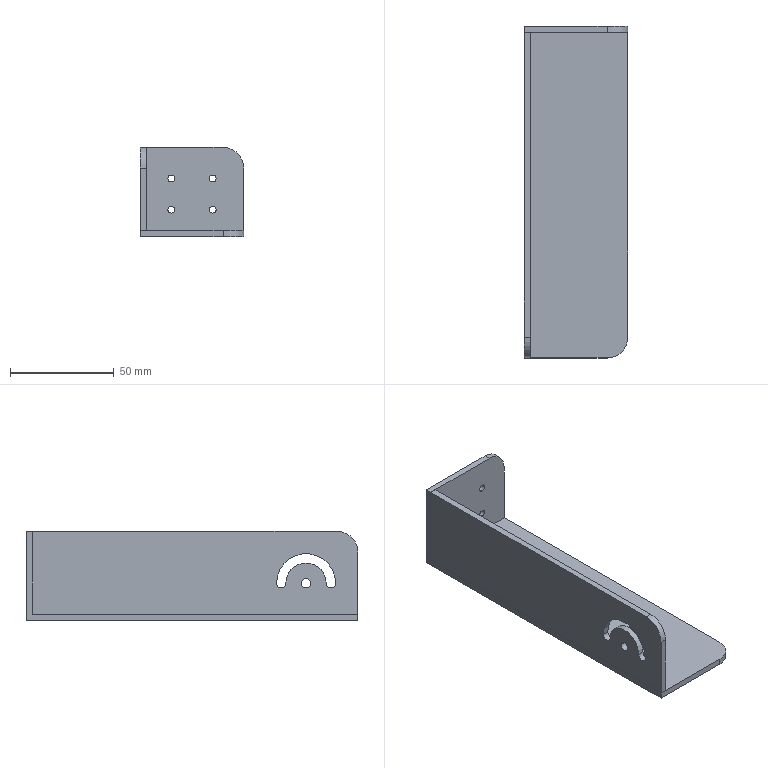Part | SolidWorks | features ICE 3, Fillet 2, Extrusion 1, HoleWzd 1 | 2 solids | 31 faces | box 50 x 160 x 43 mm | volume 47940 mm3 | cylinder 17 | plane 14 | commonest cylinder face diameters 3.3 x8 4.5 x4 20 x3 19.5 x1 28.5 x1
STEP:
#1=CARTESIAN_POINT('',(-25.,-52.75,18.));
#2=VERTEX_POINT('',#1);
#3=CARTESIAN_POINT('',(-25.,-57.25,18.));
#4=VERTEX_POINT('',#3);
#5=CARTESIAN_POINT('',(-25.,-55.,18.));
#6=DIRECTION('',(-1.,0.,0.));
#7=DIRECTION('',(0.,-1.,0.));
#8=AXIS2_PLACEMENT_3D('',#5,#6,#7);
#9=CIRCLE('',#8,2.25);
#10=EDGE_CURVE('',#2,#4,#9,.T.);
#11=ORIENTED_EDGE('',*,*,#10,.T.);
#12=CARTESIAN_POINT('',(-22.,-57.25,18.));
#13=VERTEX_POINT('',#12);
#14=CARTESIAN_POINT('',(-32.,-57.25,18.));
#15=DIRECTION('',(1.,0.,0.));
#16=VECTOR('',#15,1000.);
#17=LINE('',#14,#16);
#18=EDGE_CURVE('',#4,#13,#17,.T.);
#19=ORIENTED_EDGE('',*,*,#18,.T.);
#20=CARTESIAN_POINT('',(-22.,-52.75,18.));
#21=VERTEX_POINT('',#20);
#22=CARTESIAN_POINT('',(-22.,-55.,18.));
#23=DIRECTION('',(1.,0.,0.));
#24=DIRECTION('',(0.,1.,0.));
#25=AXIS2_PLACEMENT_3D('',#22,#23,#24);
#26=CIRCLE('',#25,2.25);
#27=EDGE_CURVE('',#13,#21,#26,.T.);
#28=ORIENTED_EDGE('',*,*,#27,.T.);
#29=CARTESIAN_POINT('',(-32.,-52.75,18.));
#30=DIRECTION('',(1.,0.,0.));
#31=VECTOR('',#30,1000.);
#32=LINE('',#29,#31);
#33=EDGE_CURVE('',#2,#21,#32,.T.);
#34=ORIENTED_EDGE('',*,*,#33,.F.);
#35=EDGE_LOOP('',(#11,#19,#28,#34));
#36=FACE_OUTER_BOUND('',#35,.T.);
#37=CARTESIAN_POINT('',(-32.,-55.,18.));
#38=DIRECTION('',(1.,0.,0.));
#39=DIRECTION('',(0.,1.,0.));
#40=AXIS2_PLACEMENT_3D('',#37,#38,#39);
#41=CYLINDRICAL_SURFACE('',#40,2.25);
#42=ADVANCED_FACE('',(#36),#41,.F.);
#43=CARTESIAN_POINT('',(-22.,-55.,18.));
#44=DIRECTION('',(1.,0.,0.));
#45=DIRECTION('',(0.,1.,0.));
#46=AXIS2_PLACEMENT_3D('',#43,#44,#45);
#47=CIRCLE('',#46,2.25);
#48=EDGE_CURVE('',#21,#13,#47,.T.);
#49=ORIENTED_EDGE('',*,*,#48,.F.);
#50=ORIENTED_EDGE('',*,*,#27,.F.);
#51=EDGE_LOOP('',(#49,#50));
#52=FACE_BOUND('',#51,.T.);
#53=CARTESIAN_POINT('',(-22.,-70.,43.));
#54=VERTEX_POINT('',#53);
#55=CARTESIAN_POINT('',(-22.,77.,43.));
#56=VERTEX_POINT('',#55);
#57=CARTESIAN_POINT('',(-22.,77.,43.));
#58=DIRECTION('',(0.,1.,0.));
#59=VECTOR('',#58,1000.);
#60=LINE('',#57,#59);
#61=EDGE_CURVE('',#54,#56,#60,.T.);
#62=ORIENTED_EDGE('',*,*,#61,.F.);
#63=CARTESIAN_POINT('',(-22.,-80.,33.));
#64=VERTEX_POINT('',#63);
#65=CARTESIAN_POINT('',(-22.,-70.,33.));
#66=DIRECTION('',(1.,0.,0.));
#67=DIRECTION('',(0.,-1.,0.));
#68=AXIS2_PLACEMENT_3D('',#65,#66,#67);
#69=CIRCLE('',#68,10.);
#70=EDGE_CURVE('',#54,#64,#69,.T.);
#71=ORIENTED_EDGE('',*,*,#70,.T.);
#72=CARTESIAN_POINT('',(-22.,-80.,3.));
#73=VERTEX_POINT('',#72);
#74=CARTESIAN_POINT('',(-22.,-80.,3.));
#75=DIRECTION('',(0.,0.,1.));
#76=VECTOR('',#75,1000.);
#77=LINE('',#74,#76);
#78=EDGE_CURVE('',#73,#64,#77,.T.);
#79=ORIENTED_EDGE('',*,*,#78,.F.);
#80=CARTESIAN_POINT('',(-22.,77.,3.));
#81=VERTEX_POINT('',#80);
#82=CARTESIAN_POINT('',(-22.,77.,3.));
#83=DIRECTION('',(0.,-1.,0.));
#84=VECTOR('',#83,1000.);
#85=LINE('',#82,#84);
#86=EDGE_CURVE('',#81,#73,#85,.T.);
#87=ORIENTED_EDGE('',*,*,#86,.F.);
#88=CARTESIAN_POINT('',(-22.,77.,3.));
#89=DIRECTION('',(0.,0.,-1.));
#90=VECTOR('',#89,1000.);
#91=LINE('',#88,#90);
#92=EDGE_CURVE('',#56,#81,#91,.T.);
#93=ORIENTED_EDGE('',*,*,#92,.F.);
#94=EDGE_LOOP('',(#62,#71,#79,#87,#93));
#95=FACE_OUTER_BOUND('',#94,.T.);
#96=CARTESIAN_POINT('',(-22.,-64.75,18.));
#97=VERTEX_POINT('',#96);
#98=CARTESIAN_POINT('',(-22.,-45.25,18.));
#99=VERTEX_POINT('',#98);
#100=CARTESIAN_POINT('',(-22.,-55.,18.));
#101=DIRECTION('',(-1.,0.,0.));
#102=DIRECTION('',(0.,1.,0.));
#103=AXIS2_PLACEMENT_3D('',#100,#101,#102);
#104=CIRCLE('',#103,9.75);
#105=EDGE_CURVE('',#97,#99,#104,.T.);
#106=ORIENTED_EDGE('',*,*,#105,.F.);
#107=CARTESIAN_POINT('',(-22.,-69.25,18.));
#108=VERTEX_POINT('',#107);
#109=CARTESIAN_POINT('',(-22.,-67.,18.));
#110=DIRECTION('',(1.,0.,0.));
#111=DIRECTION('',(0.,1.,0.));
#112=AXIS2_PLACEMENT_3D('',#109,#110,#111);
#113=CIRCLE('',#112,2.25);
#114=EDGE_CURVE('',#108,#97,#113,.T.);
#115=ORIENTED_EDGE('',*,*,#114,.F.);
#116=CARTESIAN_POINT('',(-22.,-40.75,18.));
#117=VERTEX_POINT('',#116);
#118=CARTESIAN_POINT('',(-22.,-55.,18.));
#119=DIRECTION('',(1.,0.,0.));
#120=DIRECTION('',(0.,1.,0.));
#121=AXIS2_PLACEMENT_3D('',#118,#119,#120);
#122=CIRCLE('',#121,14.25);
#123=EDGE_CURVE('',#117,#108,#122,.T.);
#124=ORIENTED_EDGE('',*,*,#123,.F.);
#125=CARTESIAN_POINT('',(-22.,-43.,18.));
#126=DIRECTION('',(1.,0.,0.));
#127=DIRECTION('',(0.,1.,0.));
#128=AXIS2_PLACEMENT_3D('',#125,#126,#127);
#129=CIRCLE('',#128,2.25);
#130=EDGE_CURVE('',#99,#117,#129,.T.);
#131=ORIENTED_EDGE('',*,*,#130,.F.);
#132=EDGE_LOOP('',(#106,#115,#124,#131));
#133=FACE_BOUND('',#132,.T.);
#134=CARTESIAN_POINT('',(-22.,0.,0.));
#135=DIRECTION('',(-1.,0.,0.));
#136=DIRECTION('',(0.,-1.,0.));
#137=AXIS2_PLACEMENT_3D('',#134,#135,#136);
#138=PLANE('',#137);
#139=ADVANCED_FACE('',(#52,#95,#133),#138,.F.);
#140=CARTESIAN_POINT('',(-25.,-80.,3.));
#141=VERTEX_POINT('',#140);
#142=CARTESIAN_POINT('',(-25.,-80.,33.));
#143=VERTEX_POINT('',#142);
#144=CARTESIAN_POINT('',(-25.,-80.,3.));
#145=DIRECTION('',(0.,0.,1.));
#146=VECTOR('',#145,1000.);
#147=LINE('',#144,#146);
#148=EDGE_CURVE('',#141,#143,#147,.T.);
#149=ORIENTED_EDGE('',*,*,#148,.T.);
#150=CARTESIAN_POINT('',(-25.,-70.,43.));
#151=VERTEX_POINT('',#150);
#152=CARTESIAN_POINT('',(-25.,-70.,33.));
#153=DIRECTION('',(-1.,0.,0.));
#154=DIRECTION('',(0.,-1.,0.));
#155=AXIS2_PLACEMENT_3D('',#152,#153,#154);
#156=CIRCLE('',#155,10.);
#157=EDGE_CURVE('',#143,#151,#156,.T.);
#158=ORIENTED_EDGE('',*,*,#157,.T.);
#159=CARTESIAN_POINT('',(-25.,77.,43.));
#160=VERTEX_POINT('',#159);
#161=CARTESIAN_POINT('',(-25.,77.,43.));
#162=DIRECTION('',(0.,1.,0.));
#163=VECTOR('',#162,1000.);
#164=LINE('',#161,#163);
#165=EDGE_CURVE('',#151,#160,#164,.T.);
#166=ORIENTED_EDGE('',*,*,#165,.T.);
#167=CARTESIAN_POINT('',(-25.,77.,3.));
#168=VERTEX_POINT('',#167);
#169=CARTESIAN_POINT('',(-25.,77.,3.));
#170=DIRECTION('',(0.,0.,-1.));
#171=VECTOR('',#170,1000.);
#172=LINE('',#169,#171);
#173=EDGE_CURVE('',#160,#168,#172,.T.);
#174=ORIENTED_EDGE('',*,*,#173,.T.);
#175=CARTESIAN_POINT('',(-25.,77.,3.));
#176=DIRECTION('',(0.,-1.,0.));
#177=VECTOR('',#176,1000.);
#178=LINE('',#175,#177);
#179=EDGE_CURVE('',#168,#141,#178,.T.);
#180=ORIENTED_EDGE('',*,*,#179,.T.);
#181=EDGE_LOOP('',(#149,#158,#166,#174,#180));
#182=FACE_OUTER_BOUND('',#181,.T.);
#183=ORIENTED_EDGE('',*,*,#10,.F.);
#184=CARTESIAN_POINT('',(-25.,-55.,18.));
#185=DIRECTION('',(-1.,0.,0.));
#186=DIRECTION('',(0.,-1.,0.));
#187=AXIS2_PLACEMENT_3D('',#184,#185,#186);
#188=CIRCLE('',#187,2.25);
#189=EDGE_CURVE('',#4,#2,#188,.T.);
#190=ORIENTED_EDGE('',*,*,#189,.F.);
#191=EDGE_LOOP('',(#183,#190));
#192=FACE_BOUND('',#191,.T.);
#193=CARTESIAN_POINT('',(-25.,-64.75,18.));
#194=VERTEX_POINT('',#193);
#195=CARTESIAN_POINT('',(-25.,-69.25,18.));
#196=VERTEX_POINT('',#195);
#197=CARTESIAN_POINT('',(-25.,-67.,18.));
#198=DIRECTION('',(-1.,0.,0.));
#199=DIRECTION('',(0.,-1.,0.));
#200=AXIS2_PLACEMENT_3D('',#197,#198,#199);
#201=CIRCLE('',#200,2.25);
#202=EDGE_CURVE('',#194,#196,#201,.T.);
#203=ORIENTED_EDGE('',*,*,#202,.F.);
#204=CARTESIAN_POINT('',(-25.,-45.25,18.));
#205=VERTEX_POINT('',#204);
#206=CARTESIAN_POINT('',(-25.,-55.,18.));
#207=DIRECTION('',(1.,0.,0.));
#208=DIRECTION('',(0.,-1.,0.));
#209=AXIS2_PLACEMENT_3D('',#206,#207,#208);
#210=CIRCLE('',#209,9.75);
#211=EDGE_CURVE('',#205,#194,#210,.T.);
#212=ORIENTED_EDGE('',*,*,#211,.F.);
#213=CARTESIAN_POINT('',(-25.,-40.75,18.));
#214=VERTEX_POINT('',#213);
#215=CARTESIAN_POINT('',(-25.,-43.,18.));
#216=DIRECTION('',(-1.,0.,0.));
#217=DIRECTION('',(0.,-1.,0.));
#218=AXIS2_PLACEMENT_3D('',#215,#216,#217);
#219=CIRCLE('',#218,2.25);
#220=EDGE_CURVE('',#214,#205,#219,.T.);
#221=ORIENTED_EDGE('',*,*,#220,.F.);
#222=CARTESIAN_POINT('',(-25.,-55.,18.));
#223=DIRECTION('',(-1.,0.,0.));
#224=DIRECTION('',(0.,-1.,0.));
#225=AXIS2_PLACEMENT_3D('',#222,#223,#224);
#226=CIRCLE('',#225,14.25);
#227=EDGE_CURVE('',#196,#214,#226,.T.);
#228=ORIENTED_EDGE('',*,*,#227,.F.);
#229=EDGE_LOOP('',(#203,#212,#221,#228));
#230=FACE_BOUND('',#229,.T.);
#231=CARTESIAN_POINT('',(-25.,0.,0.));
#232=DIRECTION('',(-1.,0.,0.));
#233=DIRECTION('',(0.,-1.,0.));
#234=AXIS2_PLACEMENT_3D('',#231,#232,#233);
#235=PLANE('',#234);
#236=ADVANCED_FACE('',(#182,#192,#230),#235,.T.);
#237=ORIENTED_EDGE('',*,*,#179,.F.);
#238=CARTESIAN_POINT('',(-22.,77.,3.));
#239=DIRECTION('',(-1.,0.,0.));
#240=VECTOR('',#239,1000.);
#241=LINE('',#238,#240);
#242=EDGE_CURVE('',#81,#168,#241,.T.);
#243=ORIENTED_EDGE('',*,*,#242,.F.);
#244=ORIENTED_EDGE('',*,*,#86,.T.);
#245=CARTESIAN_POINT('',(-22.,-80.,3.));
#246=DIRECTION('',(-1.,0.,0.));
#247=VECTOR('',#246,1000.);
#248=LINE('',#245,#247);
#249=EDGE_CURVE('',#73,#141,#248,.T.);
#250=ORIENTED_EDGE('',*,*,#249,.T.);
#251=EDGE_LOOP('',(#237,#243,#244,#250));
#252=FACE_OUTER_BOUND('',#251,.T.);
#253=CARTESIAN_POINT('',(-22.,77.,3.));
#254=DIRECTION('',(0.,0.,-1.));
#255=DIRECTION('',(0.,1.,0.));
#256=AXIS2_PLACEMENT_3D('',#253,#254,#255);
#257=PLANE('',#256);
#258=ADVANCED_FACE('',(#252),#257,.T.);
#259=ORIENTED_EDGE('',*,*,#173,.F.);
#260=CARTESIAN_POINT('',(-22.,77.,43.));
#261=DIRECTION('',(-1.,0.,0.));
#262=VECTOR('',#261,1000.);
#263=LINE('',#260,#262);
#264=EDGE_CURVE('',#56,#160,#263,.T.);
#265=ORIENTED_EDGE('',*,*,#264,.F.);
#266=ORIENTED_EDGE('',*,*,#92,.T.);
#267=ORIENTED_EDGE('',*,*,#242,.T.);
#268=EDGE_LOOP('',(#259,#265,#266,#267));
#269=FACE_OUTER_BOUND('',#268,.T.);
#270=CARTESIAN_POINT('',(-22.,77.,3.));
#271=DIRECTION('',(0.,1.,0.));
#272=DIRECTION('',(-1.,0.,0.));
#273=AXIS2_PLACEMENT_3D('',#270,#271,#272);
#274=PLANE('',#273);
#275=ADVANCED_FACE('',(#269),#274,.T.);
#276=ORIENTED_EDGE('',*,*,#165,.F.);
#277=CARTESIAN_POINT('',(-22.,-70.,43.));
#278=DIRECTION('',(1.,0.,0.));
#279=VECTOR('',#278,1000.);
#280=LINE('',#277,#279);
#281=EDGE_CURVE('',#151,#54,#280,.T.);
#282=ORIENTED_EDGE('',*,*,#281,.T.);
#283=ORIENTED_EDGE('',*,*,#61,.T.);
#284=ORIENTED_EDGE('',*,*,#264,.T.);
#285=EDGE_LOOP('',(#276,#282,#283,#284));
#286=FACE_OUTER_BOUND('',#285,.T.);
#287=CARTESIAN_POINT('',(-22.,77.,43.));
#288=DIRECTION('',(0.,0.,1.));
#289=DIRECTION('',(0.,-1.,0.));
#290=AXIS2_PLACEMENT_3D('',#287,#288,#289);
#291=PLANE('',#290);
#292=ADVANCED_FACE('',(#286),#291,.T.);
#293=ORIENTED_EDGE('',*,*,#78,.T.);
#294=CARTESIAN_POINT('',(-22.,-80.,33.));
#295=DIRECTION('',(-1.,0.,0.));
#296=VECTOR('',#295,1000.);
#297=LINE('',#294,#296);
#298=EDGE_CURVE('',#64,#143,#297,.T.);
#299=ORIENTED_EDGE('',*,*,#298,.T.);
#300=ORIENTED_EDGE('',*,*,#148,.F.);
#301=ORIENTED_EDGE('',*,*,#249,.F.);
#302=EDGE_LOOP('',(#293,#299,#300,#301));
#303=FACE_OUTER_BOUND('',#302,.T.);
#304=CARTESIAN_POINT('',(-22.,-80.,3.));
#305=DIRECTION('',(0.,-1.,0.));
#306=DIRECTION('',(1.,0.,0.));
#307=AXIS2_PLACEMENT_3D('',#304,#305,#306);
#308=PLANE('',#307);
#309=ADVANCED_FACE('',(#303),#308,.T.);
#310=ORIENTED_EDGE('',*,*,#18,.F.);
#311=ORIENTED_EDGE('',*,*,#189,.T.);
#312=ORIENTED_EDGE('',*,*,#33,.T.);
#313=ORIENTED_EDGE('',*,*,#48,.T.);
#314=EDGE_LOOP('',(#310,#311,#312,#313));
#315=FACE_OUTER_BOUND('',#314,.T.);
#316=CARTESIAN_POINT('',(-32.,-55.,18.));
#317=DIRECTION('',(1.,0.,0.));
#318=DIRECTION('',(0.,1.,0.));
#319=AXIS2_PLACEMENT_3D('',#316,#317,#318);
#320=CYLINDRICAL_SURFACE('',#319,2.25);
#321=ADVANCED_FACE('',(#315),#320,.F.);
#322=ORIENTED_EDGE('',*,*,#202,.T.);
#323=CARTESIAN_POINT('',(-32.,-69.25,18.));
#324=DIRECTION('',(1.,0.,0.));
#325=VECTOR('',#324,1000.);
#326=LINE('',#323,#325);
#327=EDGE_CURVE('',#196,#108,#326,.T.);
#328=ORIENTED_EDGE('',*,*,#327,.T.);
#329=ORIENTED_EDGE('',*,*,#114,.T.);
#330=CARTESIAN_POINT('',(-32.,-64.75,18.));
#331=DIRECTION('',(1.,0.,0.));
#332=VECTOR('',#331,1000.);
#333=LINE('',#330,#332);
#334=EDGE_CURVE('',#194,#97,#333,.T.);
#335=ORIENTED_EDGE('',*,*,#334,.F.);
#336=EDGE_LOOP('',(#322,#328,#329,#335));
#337=FACE_OUTER_BOUND('',#336,.T.);
#338=CARTESIAN_POINT('',(-32.,-67.,18.));
#339=DIRECTION('',(1.,0.,0.));
#340=DIRECTION('',(0.,1.,0.));
#341=AXIS2_PLACEMENT_3D('',#338,#339,#340);
#342=CYLINDRICAL_SURFACE('',#341,2.25);
#343=ADVANCED_FACE('',(#337),#342,.F.);
#344=ORIENTED_EDGE('',*,*,#227,.T.);
#345=CARTESIAN_POINT('',(-32.,-40.75,18.));
#346=DIRECTION('',(1.,0.,0.));
#347=VECTOR('',#346,1000.);
#348=LINE('',#345,#347);
#349=EDGE_CURVE('',#214,#117,#348,.T.);
#350=ORIENTED_EDGE('',*,*,#349,.T.);
#351=ORIENTED_EDGE('',*,*,#123,.T.);
#352=ORIENTED_EDGE('',*,*,#327,.F.);
#353=EDGE_LOOP('',(#344,#350,#351,#352));
#354=FACE_OUTER_BOUND('',#353,.T.);
#355=CARTESIAN_POINT('',(-32.,-55.,18.));
#356=DIRECTION('',(1.,0.,0.));
#357=DIRECTION('',(0.,1.,0.));
#358=AXIS2_PLACEMENT_3D('',#355,#356,#357);
#359=CYLINDRICAL_SURFACE('',#358,14.25);
#360=ADVANCED_FACE('',(#354),#359,.F.);
#361=ORIENTED_EDGE('',*,*,#220,.T.);
#362=CARTESIAN_POINT('',(-32.,-45.25,18.));
#363=DIRECTION('',(1.,0.,0.));
#364=VECTOR('',#363,1000.);
#365=LINE('',#362,#364);
#366=EDGE_CURVE('',#205,#99,#365,.T.);
#367=ORIENTED_EDGE('',*,*,#366,.T.);
#368=ORIENTED_EDGE('',*,*,#130,.T.);
#369=ORIENTED_EDGE('',*,*,#349,.F.);
#370=EDGE_LOOP('',(#361,#367,#368,#369));
#371=FACE_OUTER_BOUND('',#370,.T.);
#372=CARTESIAN_POINT('',(-32.,-43.,18.));
#373=DIRECTION('',(1.,0.,0.));
#374=DIRECTION('',(0.,1.,0.));
#375=AXIS2_PLACEMENT_3D('',#372,#373,#374);
#376=CYLINDRICAL_SURFACE('',#375,2.25);
#377=ADVANCED_FACE('',(#371),#376,.F.);
#378=ORIENTED_EDGE('',*,*,#211,.T.);
#379=ORIENTED_EDGE('',*,*,#334,.T.);
#380=ORIENTED_EDGE('',*,*,#105,.T.);
#381=ORIENTED_EDGE('',*,*,#366,.F.);
#382=EDGE_LOOP('',(#378,#379,#380,#381));
#383=FACE_OUTER_BOUND('',#382,.T.);
#384=CARTESIAN_POINT('',(-32.,-55.,18.));
#385=DIRECTION('',(1.,0.,0.));
#386=DIRECTION('',(0.,1.,0.));
#387=AXIS2_PLACEMENT_3D('',#384,#385,#386);
#388=CYLINDRICAL_SURFACE('',#387,9.75);
#389=ADVANCED_FACE('',(#383),#388,.T.);
#390=ORIENTED_EDGE('',*,*,#70,.F.);
#391=ORIENTED_EDGE('',*,*,#281,.F.);
#392=ORIENTED_EDGE('',*,*,#157,.F.);
#393=ORIENTED_EDGE('',*,*,#298,.F.);
#394=EDGE_LOOP('',(#390,#391,#392,#393));
#395=FACE_OUTER_BOUND('',#394,.T.);
#396=CARTESIAN_POINT('',(-22.,-70.,33.));
#397=DIRECTION('',(-1.,0.,0.));
#398=DIRECTION('',(0.,-1.,0.));
#399=AXIS2_PLACEMENT_3D('',#396,#397,#398);
#400=CYLINDRICAL_SURFACE('',#399,10.);
#401=ADVANCED_FACE('',(#395),#400,.T.);
#402=CLOSED_SHELL('',(#42,#139,#236,#258,#275,#292,#309,#321,#343,#360,#377,#389,#401));
#403=MANIFOLD_SOLID_BREP('',#402);
#404=CARTESIAN_POINT('',(-10.,77.,11.35));
#405=VERTEX_POINT('',#404);
#406=CARTESIAN_POINT('',(-10.,77.,14.65));
#407=VERTEX_POINT('',#406);
#408=CARTESIAN_POINT('',(-10.,77.,13.));
#409=DIRECTION('',(0.,1.,0.));
#410=DIRECTION('',(0.,0.,1.));
#411=AXIS2_PLACEMENT_3D('',#408,#409,#410);
#412=CIRCLE('',#411,1.65);
#413=EDGE_CURVE('',#405,#407,#412,.T.);
#414=ORIENTED_EDGE('',*,*,#413,.F.);
#415=CARTESIAN_POINT('',(-10.,80.,11.35));
#416=VERTEX_POINT('',#415);
#417=CARTESIAN_POINT('',(-10.,80.,11.35));
#418=DIRECTION('',(0.,1.,0.));
#419=VECTOR('',#418,1000.);
#420=LINE('',#417,#419);
#421=EDGE_CURVE('',#405,#416,#420,.T.);
#422=ORIENTED_EDGE('',*,*,#421,.T.);
#423=CARTESIAN_POINT('',(-10.,80.,14.65));
#424=VERTEX_POINT('',#423);
#425=CARTESIAN_POINT('',(-10.,80.,13.));
#426=DIRECTION('',(0.,1.,0.));
#427=DIRECTION('',(0.,0.,1.));
#428=AXIS2_PLACEMENT_3D('',#425,#426,#427);
#429=CIRCLE('',#428,1.65);
#430=EDGE_CURVE('',#416,#424,#429,.T.);
#431=ORIENTED_EDGE('',*,*,#430,.T.);
#432=CARTESIAN_POINT('',(-10.,80.,14.65));
#433=DIRECTION('',(0.,1.,0.));
#434=VECTOR('',#433,1000.);
#435=LINE('',#432,#434);
#436=EDGE_CURVE('',#407,#424,#435,.T.);
#437=ORIENTED_EDGE('',*,*,#436,.F.);
#438=EDGE_LOOP('',(#414,#422,#431,#437));
#439=FACE_OUTER_BOUND('',#438,.T.);
#440=CARTESIAN_POINT('',(-10.,80.,13.));
#441=DIRECTION('',(0.,1.,0.));
#442=DIRECTION('',(0.,0.,1.));
#443=AXIS2_PLACEMENT_3D('',#440,#441,#442);
#444=CYLINDRICAL_SURFACE('',#443,1.65);
#445=ADVANCED_FACE('',(#439),#444,.F.);
#446=CARTESIAN_POINT('',(10.,77.,11.35));
#447=VERTEX_POINT('',#446);
#448=CARTESIAN_POINT('',(10.,77.,14.65));
#449=VERTEX_POINT('',#448);
#450=CARTESIAN_POINT('',(10.,77.,13.));
#451=DIRECTION('',(0.,1.,0.));
#452=DIRECTION('',(0.,0.,1.));
#453=AXIS2_PLACEMENT_3D('',#450,#451,#452);
#454=CIRCLE('',#453,1.65);
#455=EDGE_CURVE('',#447,#449,#454,.T.);
#456=ORIENTED_EDGE('',*,*,#455,.F.);
#457=CARTESIAN_POINT('',(10.,80.,11.35));
#458=VERTEX_POINT('',#457);
#459=CARTESIAN_POINT('',(10.,80.,11.35));
#460=DIRECTION('',(0.,1.,0.));
#461=VECTOR('',#460,1000.);
#462=LINE('',#459,#461);
#463=EDGE_CURVE('',#447,#458,#462,.T.);
#464=ORIENTED_EDGE('',*,*,#463,.T.);
#465=CARTESIAN_POINT('',(10.,80.,14.65));
#466=VERTEX_POINT('',#465);
#467=CARTESIAN_POINT('',(10.,80.,13.));
#468=DIRECTION('',(0.,1.,0.));
#469=DIRECTION('',(0.,0.,1.));
#470=AXIS2_PLACEMENT_3D('',#467,#468,#469);
#471=CIRCLE('',#470,1.65);
#472=EDGE_CURVE('',#458,#466,#471,.T.);
#473=ORIENTED_EDGE('',*,*,#472,.T.);
#474=CARTESIAN_POINT('',(10.,80.,14.65));
#475=DIRECTION('',(0.,1.,0.));
#476=VECTOR('',#475,1000.);
#477=LINE('',#474,#476);
#478=EDGE_CURVE('',#449,#466,#477,.T.);
#479=ORIENTED_EDGE('',*,*,#478,.F.);
#480=EDGE_LOOP('',(#456,#464,#473,#479));
#481=FACE_OUTER_BOUND('',#480,.T.);
#482=CARTESIAN_POINT('',(10.,80.,13.));
#483=DIRECTION('',(0.,1.,0.));
#484=DIRECTION('',(0.,0.,1.));
#485=AXIS2_PLACEMENT_3D('',#482,#483,#484);
#486=CYLINDRICAL_SURFACE('',#485,1.65);
#487=ADVANCED_FACE('',(#481),#486,.F.);
#488=CARTESIAN_POINT('',(-10.,77.,26.35));
#489=VERTEX_POINT('',#488);
#490=CARTESIAN_POINT('',(-10.,77.,29.65));
#491=VERTEX_POINT('',#490);
#492=CARTESIAN_POINT('',(-10.,77.,28.));
#493=DIRECTION('',(0.,1.,0.));
#494=DIRECTION('',(0.,0.,1.));
#495=AXIS2_PLACEMENT_3D('',#492,#493,#494);
#496=CIRCLE('',#495,1.65);
#497=EDGE_CURVE('',#489,#491,#496,.T.);
#498=ORIENTED_EDGE('',*,*,#497,.F.);
#499=CARTESIAN_POINT('',(-10.,80.,26.35));
#500=VERTEX_POINT('',#499);
#501=CARTESIAN_POINT('',(-10.,80.,26.35));
#502=DIRECTION('',(0.,1.,0.));
#503=VECTOR('',#502,1000.);
#504=LINE('',#501,#503);
#505=EDGE_CURVE('',#489,#500,#504,.T.);
#506=ORIENTED_EDGE('',*,*,#505,.T.);
#507=CARTESIAN_POINT('',(-10.,80.,29.65));
#508=VERTEX_POINT('',#507);
#509=CARTESIAN_POINT('',(-10.,80.,28.));
#510=DIRECTION('',(0.,1.,0.));
#511=DIRECTION('',(0.,0.,1.));
#512=AXIS2_PLACEMENT_3D('',#509,#510,#511);
#513=CIRCLE('',#512,1.65);
#514=EDGE_CURVE('',#500,#508,#513,.T.);
#515=ORIENTED_EDGE('',*,*,#514,.T.);
#516=CARTESIAN_POINT('',(-10.,80.,29.65));
#517=DIRECTION('',(0.,1.,0.));
#518=VECTOR('',#517,1000.);
#519=LINE('',#516,#518);
#520=EDGE_CURVE('',#491,#508,#519,.T.);
#521=ORIENTED_EDGE('',*,*,#520,.F.);
#522=EDGE_LOOP('',(#498,#506,#515,#521));
#523=FACE_OUTER_BOUND('',#522,.T.);
#524=CARTESIAN_POINT('',(-10.,80.,28.));
#525=DIRECTION('',(0.,1.,0.));
#526=DIRECTION('',(0.,0.,1.));
#527=AXIS2_PLACEMENT_3D('',#524,#525,#526);
#528=CYLINDRICAL_SURFACE('',#527,1.65);
#529=ADVANCED_FACE('',(#523),#528,.F.);
#530=CARTESIAN_POINT('',(10.,77.,26.35));
#531=VERTEX_POINT('',#530);
#532=CARTESIAN_POINT('',(10.,77.,29.65));
#533=VERTEX_POINT('',#532);
#534=CARTESIAN_POINT('',(10.,77.,28.));
#535=DIRECTION('',(0.,1.,0.));
#536=DIRECTION('',(0.,0.,1.));
#537=AXIS2_PLACEMENT_3D('',#534,#535,#536);
#538=CIRCLE('',#537,1.65);
#539=EDGE_CURVE('',#531,#533,#538,.T.);
#540=ORIENTED_EDGE('',*,*,#539,.F.);
#541=CARTESIAN_POINT('',(10.,80.,26.35));
#542=VERTEX_POINT('',#541);
#543=CARTESIAN_POINT('',(10.,80.,26.35));
#544=DIRECTION('',(0.,1.,0.));
#545=VECTOR('',#544,1000.);
#546=LINE('',#543,#545);
#547=EDGE_CURVE('',#531,#542,#546,.T.);
#548=ORIENTED_EDGE('',*,*,#547,.T.);
#549=CARTESIAN_POINT('',(10.,80.,29.65));
#550=VERTEX_POINT('',#549);
#551=CARTESIAN_POINT('',(10.,80.,28.));
#552=DIRECTION('',(0.,1.,0.));
#553=DIRECTION('',(0.,0.,1.));
#554=AXIS2_PLACEMENT_3D('',#551,#552,#553);
#555=CIRCLE('',#554,1.65);
#556=EDGE_CURVE('',#542,#550,#555,.T.);
#557=ORIENTED_EDGE('',*,*,#556,.T.);
#558=CARTESIAN_POINT('',(10.,80.,29.65));
#559=DIRECTION('',(0.,1.,0.));
#560=VECTOR('',#559,1000.);
#561=LINE('',#558,#560);
#562=EDGE_CURVE('',#533,#550,#561,.T.);
#563=ORIENTED_EDGE('',*,*,#562,.F.);
#564=EDGE_LOOP('',(#540,#548,#557,#563));
#565=FACE_OUTER_BOUND('',#564,.T.);
#566=CARTESIAN_POINT('',(10.,80.,28.));
#567=DIRECTION('',(0.,1.,0.));
#568=DIRECTION('',(0.,0.,1.));
#569=AXIS2_PLACEMENT_3D('',#566,#567,#568);
#570=CYLINDRICAL_SURFACE('',#569,1.65);
#571=ADVANCED_FACE('',(#565),#570,.F.);
#572=CARTESIAN_POINT('',(25.,-70.,3.));
#573=VERTEX_POINT('',#572);
#574=CARTESIAN_POINT('',(25.,77.,3.));
#575=VERTEX_POINT('',#574);
#576=CARTESIAN_POINT('',(25.,80.,3.));
#577=DIRECTION('',(0.,1.,0.));
#578=VECTOR('',#577,1000.);
#579=LINE('',#576,#578);
#580=EDGE_CURVE('',#573,#575,#579,.T.);
#581=ORIENTED_EDGE('',*,*,#580,.F.);
#582=CARTESIAN_POINT('',(25.,-70.,0.));
#583=VERTEX_POINT('',#582);
#584=CARTESIAN_POINT('',(25.,-70.,3.));
#585=DIRECTION('',(0.,0.,-1.));
#586=VECTOR('',#585,1000.);
#587=LINE('',#584,#586);
#588=EDGE_CURVE('',#573,#583,#587,.T.);
#589=ORIENTED_EDGE('',*,*,#588,.T.);
#590=CARTESIAN_POINT('',(25.,80.,0.));
#591=VERTEX_POINT('',#590);
#592=CARTESIAN_POINT('',(25.,80.,0.));
#593=DIRECTION('',(0.,1.,0.));
#594=VECTOR('',#593,1000.);
#595=LINE('',#592,#594);
#596=EDGE_CURVE('',#583,#591,#595,.T.);
#597=ORIENTED_EDGE('',*,*,#596,.T.);
#598=CARTESIAN_POINT('',(25.,80.,33.));
#599=VERTEX_POINT('',#598);
#600=CARTESIAN_POINT('',(25.,80.,3.));
#601=DIRECTION('',(0.,0.,-1.));
#602=VECTOR('',#601,1000.);
#603=LINE('',#600,#602);
#604=EDGE_CURVE('',#599,#591,#603,.T.);
#605=ORIENTED_EDGE('',*,*,#604,.F.);
#606=CARTESIAN_POINT('',(25.,77.,33.));
#607=VERTEX_POINT('',#606);
#608=CARTESIAN_POINT('',(25.,77.,33.));
#609=DIRECTION('',(0.,-1.,0.));
#610=VECTOR('',#609,1000.);
#611=LINE('',#608,#610);
#612=EDGE_CURVE('',#599,#607,#611,.T.);
#613=ORIENTED_EDGE('',*,*,#612,.T.);
#614=CARTESIAN_POINT('',(25.,77.,43.));
#615=DIRECTION('',(0.,0.,-1.));
#616=VECTOR('',#615,1000.);
#617=LINE('',#614,#616);
#618=EDGE_CURVE('',#607,#575,#617,.T.);
#619=ORIENTED_EDGE('',*,*,#618,.T.);
#620=EDGE_LOOP('',(#581,#589,#597,#605,#613,#619));
#621=FACE_OUTER_BOUND('',#620,.T.);
#622=CARTESIAN_POINT('',(25.,80.,3.));
#623=DIRECTION('',(-1.,0.,0.));
#624=DIRECTION('',(0.,-1.,0.));
#625=AXIS2_PLACEMENT_3D('',#622,#623,#624);
#626=PLANE('',#625);
#627=ADVANCED_FACE('',(#621),#626,.F.);
#628=CARTESIAN_POINT('',(-10.,80.,13.));
#629=DIRECTION('',(0.,1.,0.));
#630=DIRECTION('',(0.,0.,1.));
#631=AXIS2_PLACEMENT_3D('',#628,#629,#630);
#632=CIRCLE('',#631,1.65);
#633=EDGE_CURVE('',#424,#416,#632,.T.);
#634=ORIENTED_EDGE('',*,*,#633,.F.);
#635=ORIENTED_EDGE('',*,*,#430,.F.);
#636=EDGE_LOOP('',(#634,#635));
#637=FACE_BOUND('',#636,.T.);
#638=CARTESIAN_POINT('',(10.,80.,13.));
#639=DIRECTION('',(0.,1.,0.));
#640=DIRECTION('',(0.,0.,1.));
#641=AXIS2_PLACEMENT_3D('',#638,#639,#640);
#642=CIRCLE('',#641,1.65);
#643=EDGE_CURVE('',#466,#458,#642,.T.);
#644=ORIENTED_EDGE('',*,*,#643,.F.);
#645=ORIENTED_EDGE('',*,*,#472,.F.);
#646=EDGE_LOOP('',(#644,#645));
#647=FACE_BOUND('',#646,.T.);
#648=CARTESIAN_POINT('',(-10.,80.,28.));
#649=DIRECTION('',(0.,1.,0.));
#650=DIRECTION('',(0.,0.,1.));
#651=AXIS2_PLACEMENT_3D('',#648,#649,#650);
#652=CIRCLE('',#651,1.65);
#653=EDGE_CURVE('',#508,#500,#652,.T.);
#654=ORIENTED_EDGE('',*,*,#653,.F.);
#655=ORIENTED_EDGE('',*,*,#514,.F.);
#656=EDGE_LOOP('',(#654,#655));
#657=FACE_BOUND('',#656,.T.);
#658=CARTESIAN_POINT('',(10.,80.,28.));
#659=DIRECTION('',(0.,1.,0.));
#660=DIRECTION('',(0.,0.,1.));
#661=AXIS2_PLACEMENT_3D('',#658,#659,#660);
#662=CIRCLE('',#661,1.65);
#663=EDGE_CURVE('',#550,#542,#662,.T.);
#664=ORIENTED_EDGE('',*,*,#663,.F.);
#665=ORIENTED_EDGE('',*,*,#556,.F.);
#666=EDGE_LOOP('',(#664,#665));
#667=FACE_BOUND('',#666,.T.);
#668=CARTESIAN_POINT('',(15.,80.,43.));
#669=VERTEX_POINT('',#668);
#670=CARTESIAN_POINT('',(-25.,80.,43.));
#671=VERTEX_POINT('',#670);
#672=CARTESIAN_POINT('',(-25.,80.,43.));
#673=DIRECTION('',(-1.,0.,0.));
#674=VECTOR('',#673,1000.);
#675=LINE('',#672,#674);
#676=EDGE_CURVE('',#669,#671,#675,.T.);
#677=ORIENTED_EDGE('',*,*,#676,.F.);
#678=CARTESIAN_POINT('',(15.,80.,33.));
#679=DIRECTION('',(0.,1.,0.));
#680=DIRECTION('',(0.,0.,-1.));
#681=AXIS2_PLACEMENT_3D('',#678,#679,#680);
#682=CIRCLE('',#681,10.);
#683=EDGE_CURVE('',#669,#599,#682,.T.);
#684=ORIENTED_EDGE('',*,*,#683,.T.);
#685=ORIENTED_EDGE('',*,*,#604,.T.);
#686=CARTESIAN_POINT('',(-25.,80.,0.));
#687=VERTEX_POINT('',#686);
#688=CARTESIAN_POINT('',(-25.,80.,0.));
#689=DIRECTION('',(-1.,0.,0.));
#690=VECTOR('',#689,1000.);
#691=LINE('',#688,#690);
#692=EDGE_CURVE('',#591,#687,#691,.T.);
#693=ORIENTED_EDGE('',*,*,#692,.T.);
#694=CARTESIAN_POINT('',(-25.,80.,3.));
#695=DIRECTION('',(0.,0.,-1.));
#696=VECTOR('',#695,1000.);
#697=LINE('',#694,#696);
#698=EDGE_CURVE('',#671,#687,#697,.T.);
#699=ORIENTED_EDGE('',*,*,#698,.F.);
#700=EDGE_LOOP('',(#677,#684,#685,#693,#699));
#701=FACE_OUTER_BOUND('',#700,.T.);
#702=CARTESIAN_POINT('',(-25.,80.,3.));
#703=DIRECTION('',(0.,-1.,0.));
#704=DIRECTION('',(0.,0.,-1.));
#705=AXIS2_PLACEMENT_3D('',#702,#703,#704);
#706=PLANE('',#705);
#707=ADVANCED_FACE('',(#637,#647,#657,#667,#701),#706,.F.);
#708=CARTESIAN_POINT('',(-25.,-80.,0.));
#709=VERTEX_POINT('',#708);
#710=CARTESIAN_POINT('',(-25.,80.,0.));
#711=DIRECTION('',(0.,-1.,0.));
#712=VECTOR('',#711,1000.);
#713=LINE('',#710,#712);
#714=EDGE_CURVE('',#687,#709,#713,.T.);
#715=ORIENTED_EDGE('',*,*,#714,.T.);
#716=CARTESIAN_POINT('',(-25.,-80.,3.));
#717=VERTEX_POINT('',#716);
#718=CARTESIAN_POINT('',(-25.,-80.,3.));
#719=DIRECTION('',(0.,0.,-1.));
#720=VECTOR('',#719,1000.);
#721=LINE('',#718,#720);
#722=EDGE_CURVE('',#717,#709,#721,.T.);
#723=ORIENTED_EDGE('',*,*,#722,.F.);
#724=CARTESIAN_POINT('',(-25.,77.,3.));
#725=VERTEX_POINT('',#724);
#726=CARTESIAN_POINT('',(-25.,80.,3.));
#727=DIRECTION('',(0.,-1.,0.));
#728=VECTOR('',#727,1000.);
#729=LINE('',#726,#728);
#730=EDGE_CURVE('',#725,#717,#729,.T.);
#731=ORIENTED_EDGE('',*,*,#730,.F.);
#732=CARTESIAN_POINT('',(-25.,77.,43.));
#733=VERTEX_POINT('',#732);
#734=CARTESIAN_POINT('',(-25.,77.,43.));
#735=DIRECTION('',(0.,0.,-1.));
#736=VECTOR('',#735,1000.);
#737=LINE('',#734,#736);
#738=EDGE_CURVE('',#733,#725,#737,.T.);
#739=ORIENTED_EDGE('',*,*,#738,.F.);
#740=CARTESIAN_POINT('',(-25.,80.,43.));
#741=DIRECTION('',(0.,-1.,0.));
#742=VECTOR('',#741,1000.);
#743=LINE('',#740,#742);
#744=EDGE_CURVE('',#671,#733,#743,.T.);
#745=ORIENTED_EDGE('',*,*,#744,.F.);
#746=ORIENTED_EDGE('',*,*,#698,.T.);
#747=EDGE_LOOP('',(#715,#723,#731,#739,#745,#746));
#748=FACE_OUTER_BOUND('',#747,.T.);
#749=CARTESIAN_POINT('',(-25.,80.,3.));
#750=DIRECTION('',(1.,0.,0.));
#751=DIRECTION('',(0.,1.,0.));
#752=AXIS2_PLACEMENT_3D('',#749,#750,#751);
#753=PLANE('',#752);
#754=ADVANCED_FACE('',(#748),#753,.F.);
#755=CARTESIAN_POINT('',(15.,-80.,0.));
#756=VERTEX_POINT('',#755);
#757=CARTESIAN_POINT('',(-25.,-80.,0.));
#758=DIRECTION('',(1.,0.,0.));
#759=VECTOR('',#758,1000.);
#760=LINE('',#757,#759);
#761=EDGE_CURVE('',#709,#756,#760,.T.);
#762=ORIENTED_EDGE('',*,*,#761,.T.);
#763=CARTESIAN_POINT('',(15.,-80.,3.));
#764=VERTEX_POINT('',#763);
#765=CARTESIAN_POINT('',(15.,-80.,3.));
#766=DIRECTION('',(0.,0.,1.));
#767=VECTOR('',#766,1000.);
#768=LINE('',#765,#767);
#769=EDGE_CURVE('',#756,#764,#768,.T.);
#770=ORIENTED_EDGE('',*,*,#769,.T.);
#771=CARTESIAN_POINT('',(-25.,-80.,3.));
#772=DIRECTION('',(1.,0.,0.));
#773=VECTOR('',#772,1000.);
#774=LINE('',#771,#773);
#775=EDGE_CURVE('',#717,#764,#774,.T.);
#776=ORIENTED_EDGE('',*,*,#775,.F.);
#777=ORIENTED_EDGE('',*,*,#722,.T.);
#778=EDGE_LOOP('',(#762,#770,#776,#777));
#779=FACE_OUTER_BOUND('',#778,.T.);
#780=CARTESIAN_POINT('',(-25.,-80.,3.));
#781=DIRECTION('',(0.,1.,0.));
#782=DIRECTION('',(0.,0.,1.));
#783=AXIS2_PLACEMENT_3D('',#780,#781,#782);
#784=PLANE('',#783);
#785=ADVANCED_FACE('',(#779),#784,.F.);
#786=ORIENTED_EDGE('',*,*,#775,.T.);
#787=CARTESIAN_POINT('',(15.,-70.,3.));
#788=DIRECTION('',(0.,0.,1.));
#789=DIRECTION('',(1.,0.,0.));
#790=AXIS2_PLACEMENT_3D('',#787,#788,#789);
#791=CIRCLE('',#790,10.);
#792=EDGE_CURVE('',#764,#573,#791,.T.);
#793=ORIENTED_EDGE('',*,*,#792,.T.);
#794=ORIENTED_EDGE('',*,*,#580,.T.);
#795=CARTESIAN_POINT('',(-25.,77.,3.));
#796=DIRECTION('',(1.,0.,0.));
#797=VECTOR('',#796,1000.);
#798=LINE('',#795,#797);
#799=EDGE_CURVE('',#725,#575,#798,.T.);
#800=ORIENTED_EDGE('',*,*,#799,.F.);
#801=ORIENTED_EDGE('',*,*,#730,.T.);
#802=EDGE_LOOP('',(#786,#793,#794,#800,#801));
#803=FACE_OUTER_BOUND('',#802,.T.);
#804=CARTESIAN_POINT('',(0.,0.,3.));
#805=DIRECTION('',(0.,0.,1.));
#806=DIRECTION('',(1.,0.,0.));
#807=AXIS2_PLACEMENT_3D('',#804,#805,#806);
#808=PLANE('',#807);
#809=ADVANCED_FACE('',(#803),#808,.T.);
#810=ORIENTED_EDGE('',*,*,#596,.F.);
#811=CARTESIAN_POINT('',(15.,-70.,0.));
#812=DIRECTION('',(0.,0.,-1.));
#813=DIRECTION('',(1.,0.,0.));
#814=AXIS2_PLACEMENT_3D('',#811,#812,#813);
#815=CIRCLE('',#814,10.);
#816=EDGE_CURVE('',#583,#756,#815,.T.);
#817=ORIENTED_EDGE('',*,*,#816,.T.);
#818=ORIENTED_EDGE('',*,*,#761,.F.);
#819=ORIENTED_EDGE('',*,*,#714,.F.);
#820=ORIENTED_EDGE('',*,*,#692,.F.);
#821=EDGE_LOOP('',(#810,#817,#818,#819,#820));
#822=FACE_OUTER_BOUND('',#821,.T.);
#823=CARTESIAN_POINT('',(0.,0.,0.));
#824=DIRECTION('',(0.,0.,1.));
#825=DIRECTION('',(1.,0.,0.));
#826=AXIS2_PLACEMENT_3D('',#823,#824,#825);
#827=PLANE('',#826);
#828=ADVANCED_FACE('',(#822),#827,.F.);
#829=CARTESIAN_POINT('',(-10.,77.,13.));
#830=DIRECTION('',(0.,1.,0.));
#831=DIRECTION('',(0.,0.,1.));
#832=AXIS2_PLACEMENT_3D('',#829,#830,#831);
#833=CIRCLE('',#832,1.65);
#834=EDGE_CURVE('',#407,#405,#833,.T.);
#835=ORIENTED_EDGE('',*,*,#834,.T.);
#836=ORIENTED_EDGE('',*,*,#413,.T.);
#837=EDGE_LOOP('',(#835,#836));
#838=FACE_BOUND('',#837,.T.);
#839=CARTESIAN_POINT('',(10.,77.,13.));
#840=DIRECTION('',(0.,1.,0.));
#841=DIRECTION('',(0.,0.,1.));
#842=AXIS2_PLACEMENT_3D('',#839,#840,#841);
#843=CIRCLE('',#842,1.65);
#844=EDGE_CURVE('',#449,#447,#843,.T.);
#845=ORIENTED_EDGE('',*,*,#844,.T.);
#846=ORIENTED_EDGE('',*,*,#455,.T.);
#847=EDGE_LOOP('',(#845,#846));
#848=FACE_BOUND('',#847,.T.);
#849=CARTESIAN_POINT('',(-10.,77.,28.));
#850=DIRECTION('',(0.,1.,0.));
#851=DIRECTION('',(0.,0.,1.));
#852=AXIS2_PLACEMENT_3D('',#849,#850,#851);
#853=CIRCLE('',#852,1.65);
#854=EDGE_CURVE('',#491,#489,#853,.T.);
#855=ORIENTED_EDGE('',*,*,#854,.T.);
#856=ORIENTED_EDGE('',*,*,#497,.T.);
#857=EDGE_LOOP('',(#855,#856));
#858=FACE_BOUND('',#857,.T.);
#859=CARTESIAN_POINT('',(10.,77.,28.));
#860=DIRECTION('',(0.,1.,0.));
#861=DIRECTION('',(0.,0.,1.));
#862=AXIS2_PLACEMENT_3D('',#859,#860,#861);
#863=CIRCLE('',#862,1.65);
#864=EDGE_CURVE('',#533,#531,#863,.T.);
#865=ORIENTED_EDGE('',*,*,#864,.T.);
#866=ORIENTED_EDGE('',*,*,#539,.T.);
#867=EDGE_LOOP('',(#865,#866));
#868=FACE_BOUND('',#867,.T.);
#869=ORIENTED_EDGE('',*,*,#618,.F.);
#870=CARTESIAN_POINT('',(15.,77.,43.));
#871=VERTEX_POINT('',#870);
#872=CARTESIAN_POINT('',(15.,77.,33.));
#873=DIRECTION('',(0.,-1.,0.));
#874=DIRECTION('',(0.,0.,1.));
#875=AXIS2_PLACEMENT_3D('',#872,#873,#874);
#876=CIRCLE('',#875,10.);
#877=EDGE_CURVE('',#607,#871,#876,.T.);
#878=ORIENTED_EDGE('',*,*,#877,.T.);
#879=CARTESIAN_POINT('',(-25.,77.,43.));
#880=DIRECTION('',(1.,0.,0.));
#881=VECTOR('',#880,1000.);
#882=LINE('',#879,#881);
#883=EDGE_CURVE('',#733,#871,#882,.T.);
#884=ORIENTED_EDGE('',*,*,#883,.F.);
#885=ORIENTED_EDGE('',*,*,#738,.T.);
#886=ORIENTED_EDGE('',*,*,#799,.T.);
#887=EDGE_LOOP('',(#869,#878,#884,#885,#886));
#888=FACE_OUTER_BOUND('',#887,.T.);
#889=CARTESIAN_POINT('',(-25.,77.,43.));
#890=DIRECTION('',(0.,1.,0.));
#891=DIRECTION('',(0.,0.,1.));
#892=AXIS2_PLACEMENT_3D('',#889,#890,#891);
#893=PLANE('',#892);
#894=ADVANCED_FACE('',(#838,#848,#858,#868,#888),#893,.F.);
#895=ORIENTED_EDGE('',*,*,#883,.T.);
#896=CARTESIAN_POINT('',(15.,80.,43.));
#897=DIRECTION('',(0.,1.,0.));
#898=VECTOR('',#897,1000.);
#899=LINE('',#896,#898);
#900=EDGE_CURVE('',#871,#669,#899,.T.);
#901=ORIENTED_EDGE('',*,*,#900,.T.);
#902=ORIENTED_EDGE('',*,*,#676,.T.);
#903=ORIENTED_EDGE('',*,*,#744,.T.);
#904=EDGE_LOOP('',(#895,#901,#902,#903));
#905=FACE_OUTER_BOUND('',#904,.T.);
#906=CARTESIAN_POINT('',(0.,0.,43.));
#907=DIRECTION('',(0.,0.,1.));
#908=DIRECTION('',(1.,0.,0.));
#909=AXIS2_PLACEMENT_3D('',#906,#907,#908);
#910=PLANE('',#909);
#911=ADVANCED_FACE('',(#905),#910,.T.);
#912=ORIENTED_EDGE('',*,*,#547,.F.);
#913=ORIENTED_EDGE('',*,*,#864,.F.);
#914=ORIENTED_EDGE('',*,*,#562,.T.);
#915=ORIENTED_EDGE('',*,*,#663,.T.);
#916=EDGE_LOOP('',(#912,#913,#914,#915));
#917=FACE_OUTER_BOUND('',#916,.T.);
#918=CARTESIAN_POINT('',(10.,80.,28.));
#919=DIRECTION('',(0.,1.,0.));
#920=DIRECTION('',(0.,0.,1.));
#921=AXIS2_PLACEMENT_3D('',#918,#919,#920);
#922=CYLINDRICAL_SURFACE('',#921,1.65);
#923=ADVANCED_FACE('',(#917),#922,.F.);
#924=ORIENTED_EDGE('',*,*,#505,.F.);
#925=ORIENTED_EDGE('',*,*,#854,.F.);
#926=ORIENTED_EDGE('',*,*,#520,.T.);
#927=ORIENTED_EDGE('',*,*,#653,.T.);
#928=EDGE_LOOP('',(#924,#925,#926,#927));
#929=FACE_OUTER_BOUND('',#928,.T.);
#930=CARTESIAN_POINT('',(-10.,80.,28.));
#931=DIRECTION('',(0.,1.,0.));
#932=DIRECTION('',(0.,0.,1.));
#933=AXIS2_PLACEMENT_3D('',#930,#931,#932);
#934=CYLINDRICAL_SURFACE('',#933,1.65);
#935=ADVANCED_FACE('',(#929),#934,.F.);
#936=ORIENTED_EDGE('',*,*,#463,.F.);
#937=ORIENTED_EDGE('',*,*,#844,.F.);
#938=ORIENTED_EDGE('',*,*,#478,.T.);
#939=ORIENTED_EDGE('',*,*,#643,.T.);
#940=EDGE_LOOP('',(#936,#937,#938,#939));
#941=FACE_OUTER_BOUND('',#940,.T.);
#942=CARTESIAN_POINT('',(10.,80.,13.));
#943=DIRECTION('',(0.,1.,0.));
#944=DIRECTION('',(0.,0.,1.));
#945=AXIS2_PLACEMENT_3D('',#942,#943,#944);
#946=CYLINDRICAL_SURFACE('',#945,1.65);
#947=ADVANCED_FACE('',(#941),#946,.F.);
#948=ORIENTED_EDGE('',*,*,#421,.F.);
#949=ORIENTED_EDGE('',*,*,#834,.F.);
#950=ORIENTED_EDGE('',*,*,#436,.T.);
#951=ORIENTED_EDGE('',*,*,#633,.T.);
#952=EDGE_LOOP('',(#948,#949,#950,#951));
#953=FACE_OUTER_BOUND('',#952,.T.);
#954=CARTESIAN_POINT('',(-10.,80.,13.));
#955=DIRECTION('',(0.,1.,0.));
#956=DIRECTION('',(0.,0.,1.));
#957=AXIS2_PLACEMENT_3D('',#954,#955,#956);
#958=CYLINDRICAL_SURFACE('',#957,1.65);
#959=ADVANCED_FACE('',(#953),#958,.F.);
#960=ORIENTED_EDGE('',*,*,#792,.F.);
#961=ORIENTED_EDGE('',*,*,#769,.F.);
#962=ORIENTED_EDGE('',*,*,#816,.F.);
#963=ORIENTED_EDGE('',*,*,#588,.F.);
#964=EDGE_LOOP('',(#960,#961,#962,#963));
#965=FACE_OUTER_BOUND('',#964,.T.);
#966=CARTESIAN_POINT('',(15.,-70.,3.));
#967=DIRECTION('',(0.,0.,-1.));
#968=DIRECTION('',(-1.,0.,0.));
#969=AXIS2_PLACEMENT_3D('',#966,#967,#968);
#970=CYLINDRICAL_SURFACE('',#969,10.);
#971=ADVANCED_FACE('',(#965),#970,.T.);
#972=ORIENTED_EDGE('',*,*,#877,.F.);
#973=ORIENTED_EDGE('',*,*,#612,.F.);
#974=ORIENTED_EDGE('',*,*,#683,.F.);
#975=ORIENTED_EDGE('',*,*,#900,.F.);
#976=EDGE_LOOP('',(#972,#973,#974,#975));
#977=FACE_OUTER_BOUND('',#976,.T.);
#978=CARTESIAN_POINT('',(15.,0.,33.));
#979=DIRECTION('',(0.,-1.,0.));
#980=DIRECTION('',(1.,0.,0.));
#981=AXIS2_PLACEMENT_3D('',#978,#979,#980);
#982=CYLINDRICAL_SURFACE('',#981,10.);
#983=ADVANCED_FACE('',(#977),#982,.T.);
#984=CLOSED_SHELL('',(#445,#487,#529,#571,#627,#707,#754,#785,#809,#828,#894,#911,#923,#935,#947,#959,#971,#983));
#985=MANIFOLD_SOLID_BREP('',#984);
#986=CARTESIAN_POINT('',(0.,0.,0.));
#987=DIRECTION('',(0.,0.,1.));
#988=DIRECTION('',(1.,0.,0.));
#989=AXIS2_PLACEMENT_3D('',#986,#987,#988);
#990=(LENGTH_UNIT()NAMED_UNIT(*)SI_UNIT(.MILLI.,.METRE.));
#991=UNCERTAINTY_MEASURE_WITH_UNIT(LENGTH_MEASURE(0.00001),#990,'','');
#992=(NAMED_UNIT(*)PLANE_ANGLE_UNIT()SI_UNIT($,.RADIAN.));
#993=(NAMED_UNIT(*)SI_UNIT($,.STERADIAN.)SOLID_ANGLE_UNIT());
#994=(GEOMETRIC_REPRESENTATION_CONTEXT(3)GLOBAL_UNCERTAINTY_ASSIGNED_CONTEXT((#991))GLOBAL_UNIT_ASSIGNED_CONTEXT((#990,#992,#993))REPRESENTATION_CONTEXT('',''));
#995=ADVANCED_BREP_SHAPE_REPRESENTATION('',(#403,#985,#989),#994);